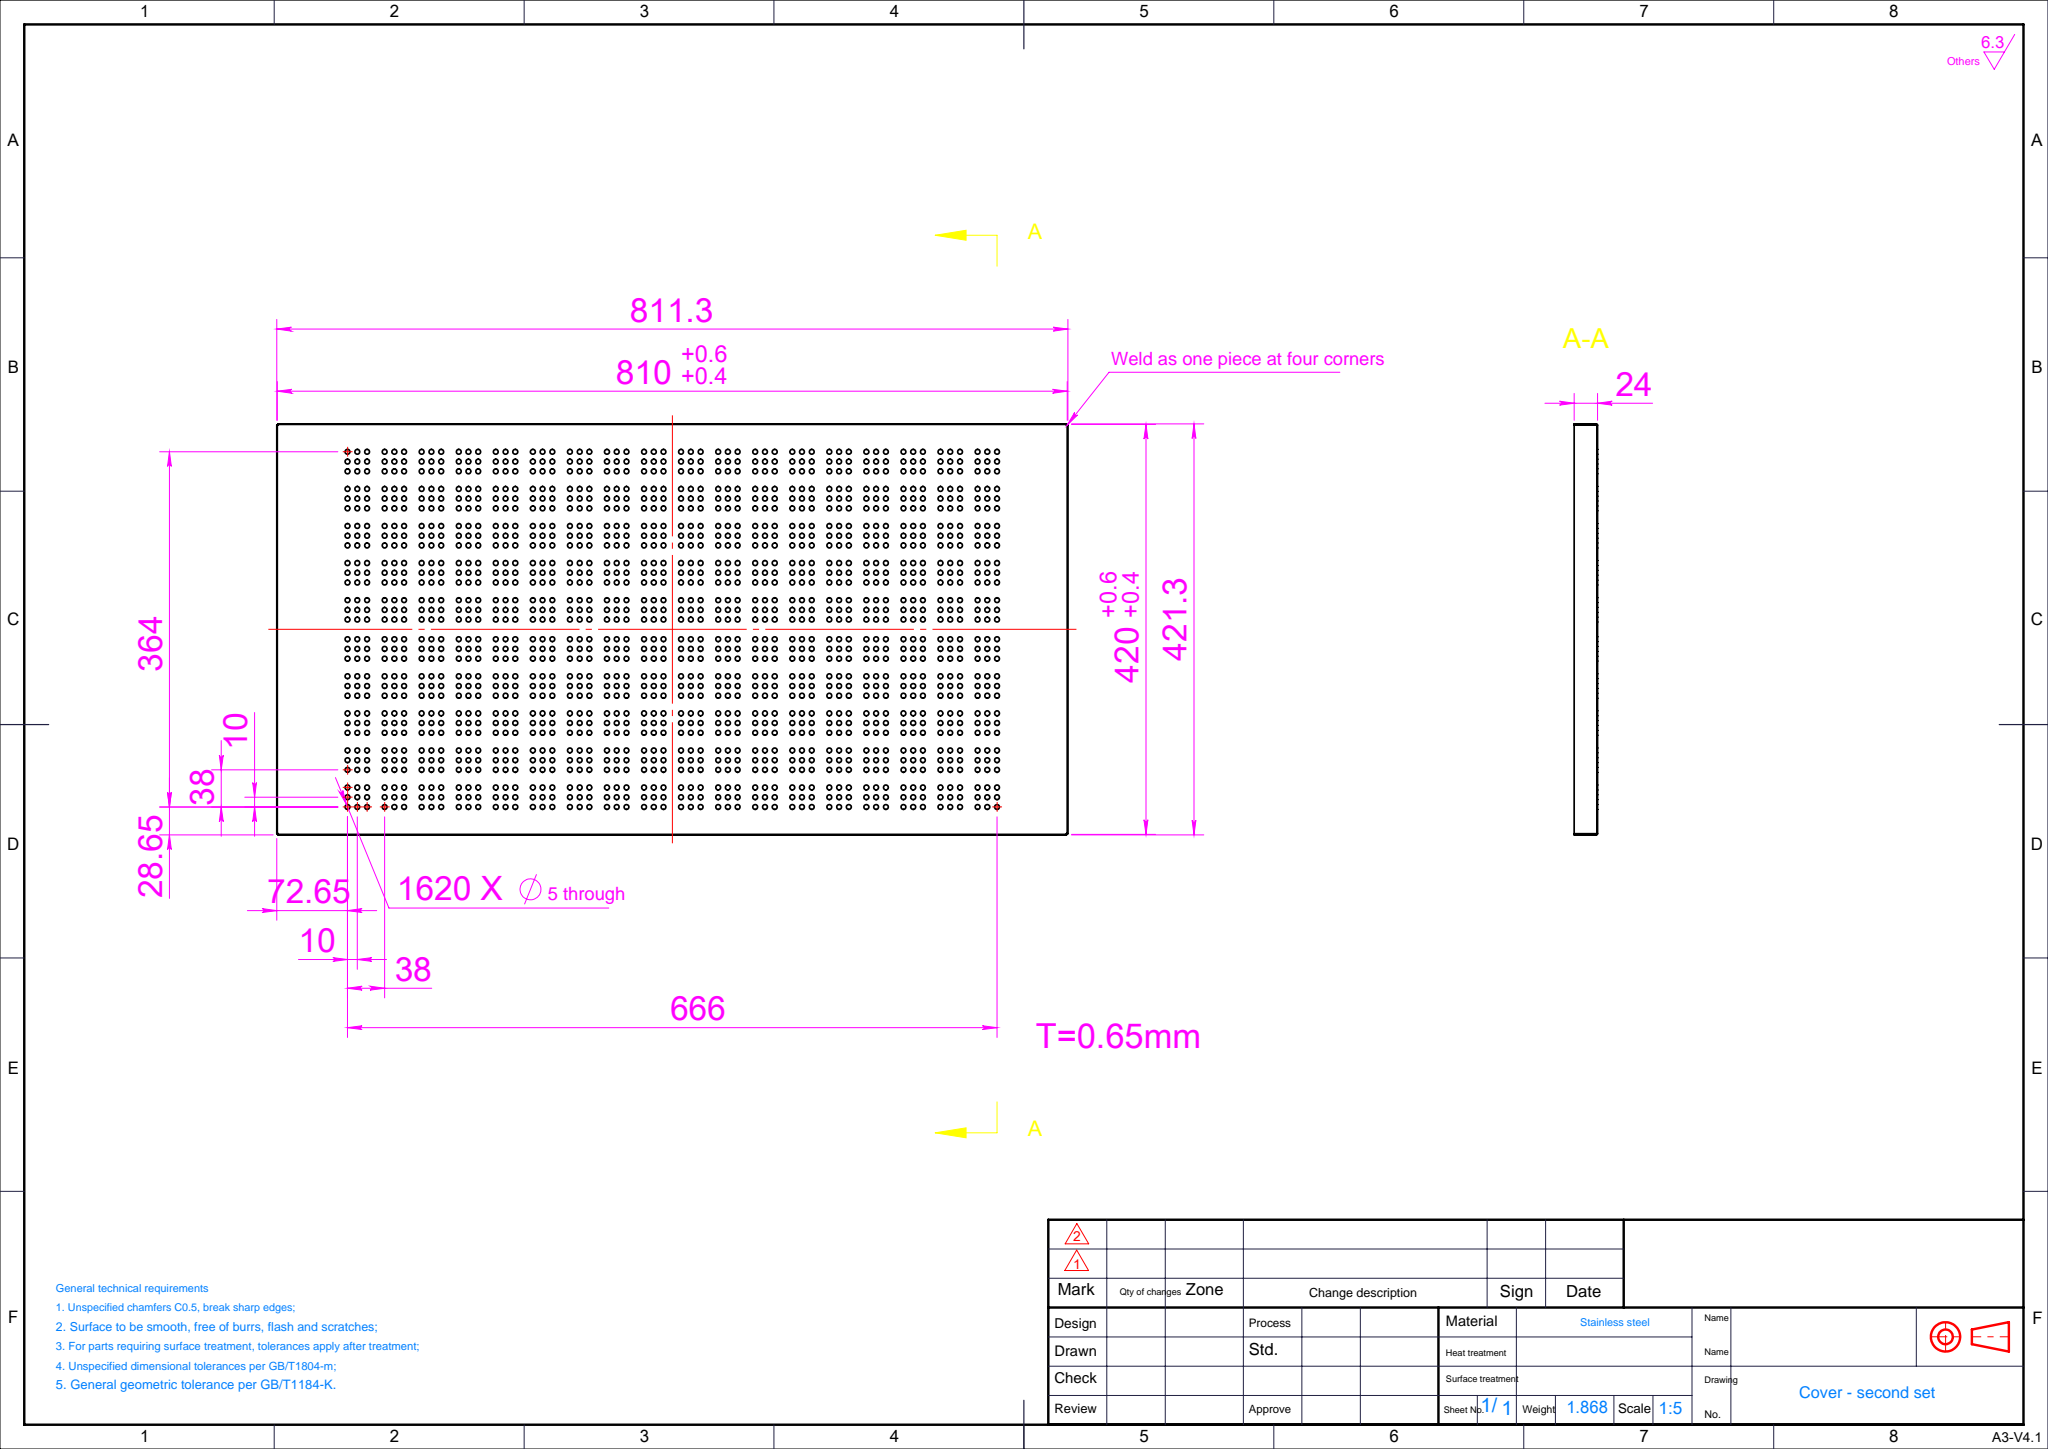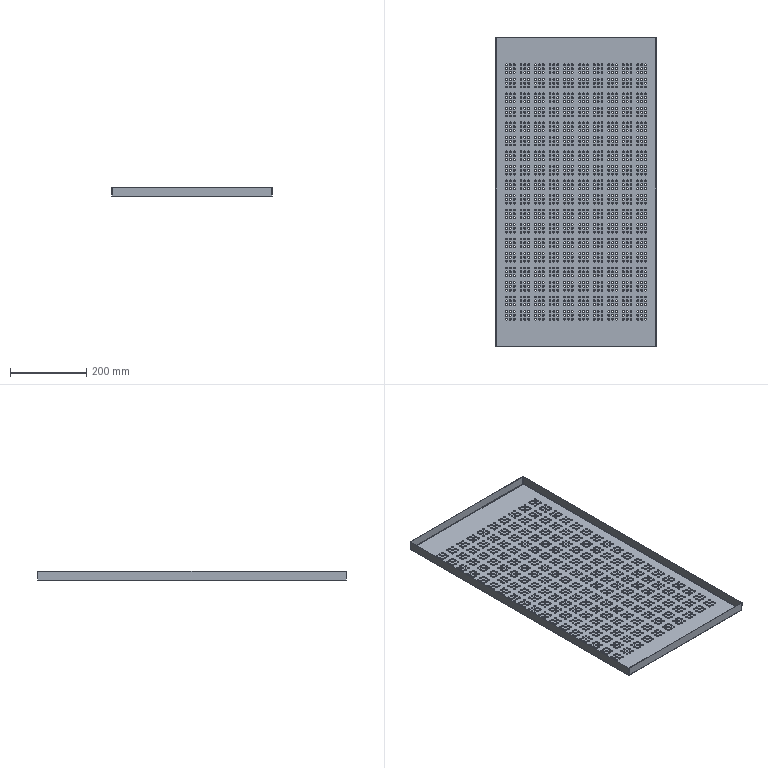Part | SolidWorks | features 3DProfileFeature 3, HoleWzd 3, LPattern 3, MirrorPattern 3, EdgeFlange 1, FlatPattern 1, SMBaseFlange 1, SheetMetal 1 | 1 solid | 3278 faces | volume 238014 mm3 | cylinder 3248 | plane 22 | spline 8 | commonest cylinder face diameters 5 x3240 1.473 x4 2.773 x4